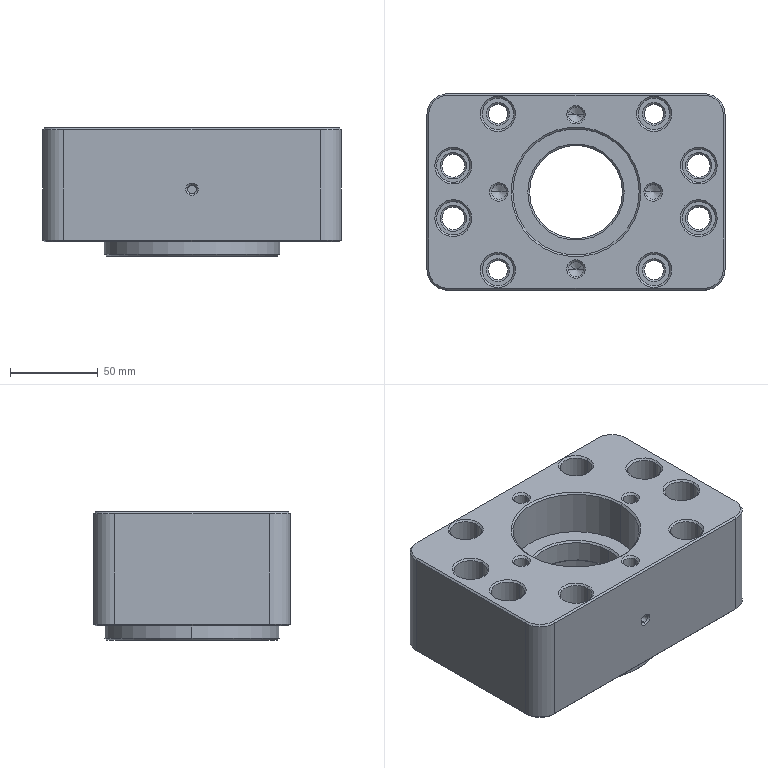NC program | NX | posted with a generic post | part box 170 x 112 x 73 mm
Lines 1 to 31 of 12427:
N10 G17 G21 G94 G90
(DRILLING_COPY , TOOL : ZXZ)
N12 T01 M6
N14 G54
N16 G17 G0 G90 X42.426 Y-15. S5000 M3
N18 G43 Z30. H1
N20 G94 G81 G98 Z-1. F250. R3.
N22 Y15.
N24 X-42.426
N26 Y-15.
N28 G80
N30 G0 X-42.426 Y-15. Z30.
N32 M5
(DRILLING_COPY_COPY_1_COPY_1 , TOOL : 3.3ZT)
N34 T13 M6
N36 G54
N38 G17 G0 G90 X42.426 Y-15. S2000 M3
N40 G43 Z30. H13
N42 G94 G83 G98 Z-14.491 F120. Q2. R3.
N44 Y15.
N46 X-42.426
N48 Y-15.
N50 G80
N52 G0 X-42.426 Y-15. Z30.
N54 M5